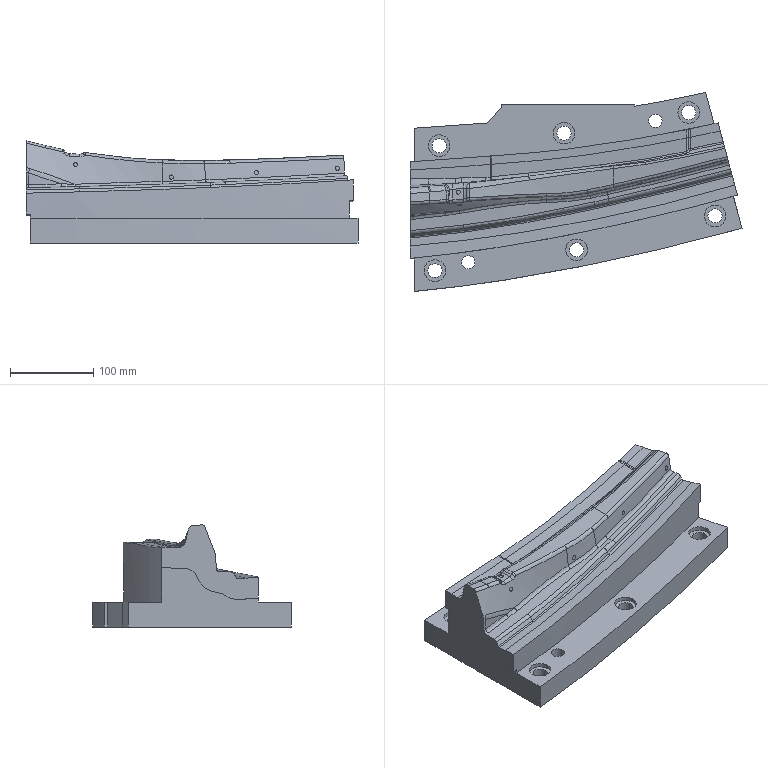Part | NX | features solid 2 | 1 solid | 143 faces | box 398.745 x 238.906 x 122.628 mm | volume 4298635 mm3 | spline 114 | plane 15 | cylinder 14 | commonest cylinder face diameters 17 x6 26 x6 16 x2